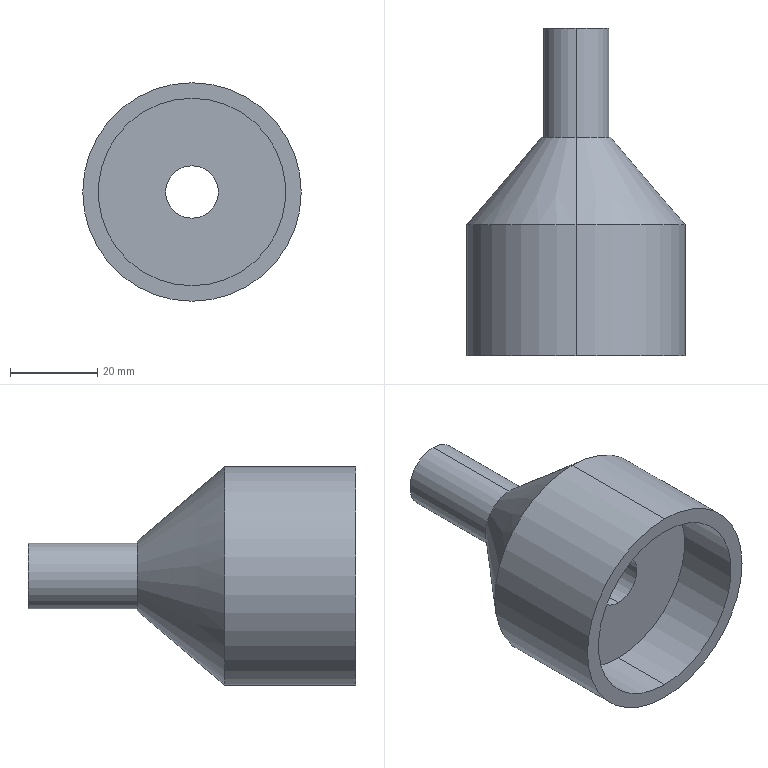Part | SolidWorks | features ICE 3, Chamfer 1, Extrusion 1 | 1 solid | 14 faces | box 50 x 75 x 50 mm | volume 53467 mm3 | cylinder 8 | plane 4 | cone 2 | commonest cylinder face diameters 12 x2 15 x2 42.907 x2 50 x2
STEP:
#1=CARTESIAN_POINT('',(0.,15.,21.453));
#2=VERTEX_POINT('',#1);
#3=CARTESIAN_POINT('',(0.,15.,-21.453));
#4=VERTEX_POINT('',#3);
#5=CARTESIAN_POINT('',(0.,15.,0.));
#6=DIRECTION('',(0.,-1.,0.));
#7=DIRECTION('',(0.,0.,-1.));
#8=AXIS2_PLACEMENT_3D('',#5,#6,#7);
#9=CIRCLE('',#8,21.453);
#10=EDGE_CURVE('',#2,#4,#9,.T.);
#11=ORIENTED_EDGE('',*,*,#10,.F.);
#12=CARTESIAN_POINT('',(0.,0.,21.453));
#13=VERTEX_POINT('',#12);
#14=CARTESIAN_POINT('',(0.,15.,21.453));
#15=DIRECTION('',(0.,-1.,0.));
#16=VECTOR('',#15,1000.);
#17=LINE('',#14,#16);
#18=EDGE_CURVE('',#2,#13,#17,.T.);
#19=ORIENTED_EDGE('',*,*,#18,.T.);
#20=CARTESIAN_POINT('',(0.,0.,-21.453));
#21=VERTEX_POINT('',#20);
#22=CARTESIAN_POINT('',(0.,0.,0.));
#23=DIRECTION('',(0.,-1.,0.));
#24=DIRECTION('',(0.,0.,-1.));
#25=AXIS2_PLACEMENT_3D('',#22,#23,#24);
#26=CIRCLE('',#25,21.453);
#27=EDGE_CURVE('',#13,#21,#26,.T.);
#28=ORIENTED_EDGE('',*,*,#27,.T.);
#29=CARTESIAN_POINT('',(0.,15.,-21.453));
#30=DIRECTION('',(0.,-1.,0.));
#31=VECTOR('',#30,1000.);
#32=LINE('',#29,#31);
#33=EDGE_CURVE('',#4,#21,#32,.T.);
#34=ORIENTED_EDGE('',*,*,#33,.F.);
#35=EDGE_LOOP('',(#11,#19,#28,#34));
#36=FACE_OUTER_BOUND('',#35,.T.);
#37=CARTESIAN_POINT('',(0.,15.,0.));
#38=DIRECTION('',(0.,-1.,0.));
#39=DIRECTION('',(0.,0.,-1.));
#40=AXIS2_PLACEMENT_3D('',#37,#38,#39);
#41=CYLINDRICAL_SURFACE('',#40,21.453);
#42=ADVANCED_FACE('',(#36),#41,.F.);
#43=CARTESIAN_POINT('',(0.,50.,8.));
#44=VERTEX_POINT('',#43);
#45=CARTESIAN_POINT('',(0.,50.,-8.));
#46=VERTEX_POINT('',#45);
#47=CARTESIAN_POINT('',(0.,50.,0.));
#48=DIRECTION('',(0.,1.,0.));
#49=DIRECTION('',(0.,0.,1.));
#50=AXIS2_PLACEMENT_3D('',#47,#48,#49);
#51=CIRCLE('',#50,8.);
#52=EDGE_CURVE('',#44,#46,#51,.T.);
#53=ORIENTED_EDGE('',*,*,#52,.F.);
#54=CARTESIAN_POINT('',(0.,30.,25.));
#55=VERTEX_POINT('',#54);
#56=CARTESIAN_POINT('',(0.,50.,8.));
#57=DIRECTION('',(0.,-0.7619,0.6476));
#58=VECTOR('',#57,1000.);
#59=LINE('',#56,#58);
#60=EDGE_CURVE('',#44,#55,#59,.T.);
#61=ORIENTED_EDGE('',*,*,#60,.T.);
#62=CARTESIAN_POINT('',(0.,30.,-25.));
#63=VERTEX_POINT('',#62);
#64=CARTESIAN_POINT('',(0.,30.,0.));
#65=DIRECTION('',(0.,-1.,0.));
#66=DIRECTION('',(0.,0.,1.));
#67=AXIS2_PLACEMENT_3D('',#64,#65,#66);
#68=CIRCLE('',#67,25.);
#69=EDGE_CURVE('',#63,#55,#68,.T.);
#70=ORIENTED_EDGE('',*,*,#69,.F.);
#71=CARTESIAN_POINT('',(0.,50.,-8.));
#72=DIRECTION('',(0.,-0.7619,-0.6476));
#73=VECTOR('',#72,1000.);
#74=LINE('',#71,#73);
#75=EDGE_CURVE('',#46,#63,#74,.T.);
#76=ORIENTED_EDGE('',*,*,#75,.F.);
#77=EDGE_LOOP('',(#53,#61,#70,#76));
#78=FACE_OUTER_BOUND('',#77,.T.);
#79=CARTESIAN_POINT('',(0.,50.,0.));
#80=DIRECTION('',(0.,-1.,0.));
#81=DIRECTION('',(0.,0.,-1.));
#82=AXIS2_PLACEMENT_3D('',#79,#80,#81);
#83=CONICAL_SURFACE('',#82,8.,0.7045);
#84=ADVANCED_FACE('',(#78),#83,.T.);
#85=CARTESIAN_POINT('',(0.,75.,7.5));
#86=VERTEX_POINT('',#85);
#87=CARTESIAN_POINT('',(0.,75.,-7.5));
#88=VERTEX_POINT('',#87);
#89=CARTESIAN_POINT('',(0.,75.,0.));
#90=DIRECTION('',(0.,1.,0.));
#91=DIRECTION('',(0.,0.,1.));
#92=AXIS2_PLACEMENT_3D('',#89,#90,#91);
#93=CIRCLE('',#92,7.5);
#94=EDGE_CURVE('',#86,#88,#93,.T.);
#95=ORIENTED_EDGE('',*,*,#94,.F.);
#96=CARTESIAN_POINT('',(0.,50.,7.5));
#97=VERTEX_POINT('',#96);
#98=CARTESIAN_POINT('',(0.,75.,7.5));
#99=DIRECTION('',(0.,-1.,0.));
#100=VECTOR('',#99,1000.);
#101=LINE('',#98,#100);
#102=EDGE_CURVE('',#86,#97,#101,.T.);
#103=ORIENTED_EDGE('',*,*,#102,.T.);
#104=CARTESIAN_POINT('',(0.,50.,-7.5));
#105=VERTEX_POINT('',#104);
#106=CARTESIAN_POINT('',(0.,50.,0.));
#107=DIRECTION('',(0.,1.,0.));
#108=DIRECTION('',(0.,0.,1.));
#109=AXIS2_PLACEMENT_3D('',#106,#107,#108);
#110=CIRCLE('',#109,7.5);
#111=EDGE_CURVE('',#97,#105,#110,.T.);
#112=ORIENTED_EDGE('',*,*,#111,.T.);
#113=CARTESIAN_POINT('',(0.,75.,-7.5));
#114=DIRECTION('',(0.,-1.,0.));
#115=VECTOR('',#114,1000.);
#116=LINE('',#113,#115);
#117=EDGE_CURVE('',#88,#105,#116,.T.);
#118=ORIENTED_EDGE('',*,*,#117,.F.);
#119=EDGE_LOOP('',(#95,#103,#112,#118));
#120=FACE_OUTER_BOUND('',#119,.T.);
#121=CARTESIAN_POINT('',(0.,75.,0.));
#122=DIRECTION('',(0.,-1.,0.));
#123=DIRECTION('',(0.,0.,-1.));
#124=AXIS2_PLACEMENT_3D('',#121,#122,#123);
#125=CYLINDRICAL_SURFACE('',#124,7.5);
#126=ADVANCED_FACE('',(#120),#125,.T.);
#127=ORIENTED_EDGE('',*,*,#69,.T.);
#128=CARTESIAN_POINT('',(0.,0.,25.));
#129=VERTEX_POINT('',#128);
#130=CARTESIAN_POINT('',(0.,50.,25.));
#131=DIRECTION('',(0.,-1.,0.));
#132=VECTOR('',#131,1000.);
#133=LINE('',#130,#132);
#134=EDGE_CURVE('',#55,#129,#133,.T.);
#135=ORIENTED_EDGE('',*,*,#134,.T.);
#136=CARTESIAN_POINT('',(0.,0.,-25.));
#137=VERTEX_POINT('',#136);
#138=CARTESIAN_POINT('',(0.,0.,0.));
#139=DIRECTION('',(0.,1.,0.));
#140=DIRECTION('',(0.,0.,1.));
#141=AXIS2_PLACEMENT_3D('',#138,#139,#140);
#142=CIRCLE('',#141,25.);
#143=EDGE_CURVE('',#129,#137,#142,.T.);
#144=ORIENTED_EDGE('',*,*,#143,.T.);
#145=CARTESIAN_POINT('',(0.,50.,-25.));
#146=DIRECTION('',(0.,-1.,0.));
#147=VECTOR('',#146,1000.);
#148=LINE('',#145,#147);
#149=EDGE_CURVE('',#63,#137,#148,.T.);
#150=ORIENTED_EDGE('',*,*,#149,.F.);
#151=EDGE_LOOP('',(#127,#135,#144,#150));
#152=FACE_OUTER_BOUND('',#151,.T.);
#153=CARTESIAN_POINT('',(0.,50.,0.));
#154=DIRECTION('',(0.,-1.,0.));
#155=DIRECTION('',(0.,0.,-1.));
#156=AXIS2_PLACEMENT_3D('',#153,#154,#155);
#157=CYLINDRICAL_SURFACE('',#156,25.);
#158=ADVANCED_FACE('',(#152),#157,.T.);
#159=CARTESIAN_POINT('',(0.,15.,-6.));
#160=VERTEX_POINT('',#159);
#161=CARTESIAN_POINT('',(0.,15.,6.));
#162=VERTEX_POINT('',#161);
#163=CARTESIAN_POINT('',(0.,15.,0.));
#164=DIRECTION('',(0.,1.,0.));
#165=DIRECTION('',(0.,0.,-1.));
#166=AXIS2_PLACEMENT_3D('',#163,#164,#165);
#167=CIRCLE('',#166,6.);
#168=EDGE_CURVE('',#160,#162,#167,.T.);
#169=ORIENTED_EDGE('',*,*,#168,.F.);
#170=CARTESIAN_POINT('',(0.,75.,-6.));
#171=VERTEX_POINT('',#170);
#172=CARTESIAN_POINT('',(0.,0.,-6.));
#173=DIRECTION('',(0.,1.,0.));
#174=VECTOR('',#173,1000.);
#175=LINE('',#172,#174);
#176=EDGE_CURVE('',#160,#171,#175,.T.);
#177=ORIENTED_EDGE('',*,*,#176,.T.);
#178=CARTESIAN_POINT('',(0.,75.,6.));
#179=VERTEX_POINT('',#178);
#180=CARTESIAN_POINT('',(0.,75.,0.));
#181=DIRECTION('',(0.,1.,0.));
#182=DIRECTION('',(0.,0.,1.));
#183=AXIS2_PLACEMENT_3D('',#180,#181,#182);
#184=CIRCLE('',#183,6.);
#185=EDGE_CURVE('',#171,#179,#184,.T.);
#186=ORIENTED_EDGE('',*,*,#185,.T.);
#187=CARTESIAN_POINT('',(0.,0.,6.));
#188=DIRECTION('',(0.,1.,0.));
#189=VECTOR('',#188,1000.);
#190=LINE('',#187,#189);
#191=EDGE_CURVE('',#162,#179,#190,.T.);
#192=ORIENTED_EDGE('',*,*,#191,.F.);
#193=EDGE_LOOP('',(#169,#177,#186,#192));
#194=FACE_OUTER_BOUND('',#193,.T.);
#195=CARTESIAN_POINT('',(0.,0.,0.));
#196=DIRECTION('',(0.,1.,0.));
#197=DIRECTION('',(0.,0.,1.));
#198=AXIS2_PLACEMENT_3D('',#195,#196,#197);
#199=CYLINDRICAL_SURFACE('',#198,6.);
#200=ADVANCED_FACE('',(#194),#199,.F.);
#201=ORIENTED_EDGE('',*,*,#176,.F.);
#202=CARTESIAN_POINT('',(0.,15.,0.));
#203=DIRECTION('',(0.,1.,0.));
#204=DIRECTION('',(0.,0.,-1.));
#205=AXIS2_PLACEMENT_3D('',#202,#203,#204);
#206=CIRCLE('',#205,6.);
#207=EDGE_CURVE('',#162,#160,#206,.T.);
#208=ORIENTED_EDGE('',*,*,#207,.F.);
#209=ORIENTED_EDGE('',*,*,#191,.T.);
#210=CARTESIAN_POINT('',(0.,75.,0.));
#211=DIRECTION('',(0.,1.,0.));
#212=DIRECTION('',(0.,0.,1.));
#213=AXIS2_PLACEMENT_3D('',#210,#211,#212);
#214=CIRCLE('',#213,6.);
#215=EDGE_CURVE('',#179,#171,#214,.T.);
#216=ORIENTED_EDGE('',*,*,#215,.T.);
#217=EDGE_LOOP('',(#201,#208,#209,#216));
#218=FACE_OUTER_BOUND('',#217,.T.);
#219=CARTESIAN_POINT('',(0.,0.,0.));
#220=DIRECTION('',(0.,1.,0.));
#221=DIRECTION('',(0.,0.,1.));
#222=AXIS2_PLACEMENT_3D('',#219,#220,#221);
#223=CYLINDRICAL_SURFACE('',#222,6.);
#224=ADVANCED_FACE('',(#218),#223,.F.);
#225=ORIENTED_EDGE('',*,*,#134,.F.);
#226=CARTESIAN_POINT('',(0.,30.,0.));
#227=DIRECTION('',(0.,-1.,0.));
#228=DIRECTION('',(0.,0.,1.));
#229=AXIS2_PLACEMENT_3D('',#226,#227,#228);
#230=CIRCLE('',#229,25.);
#231=EDGE_CURVE('',#55,#63,#230,.T.);
#232=ORIENTED_EDGE('',*,*,#231,.T.);
#233=ORIENTED_EDGE('',*,*,#149,.T.);
#234=CARTESIAN_POINT('',(0.,0.,0.));
#235=DIRECTION('',(0.,1.,0.));
#236=DIRECTION('',(0.,0.,1.));
#237=AXIS2_PLACEMENT_3D('',#234,#235,#236);
#238=CIRCLE('',#237,25.);
#239=EDGE_CURVE('',#137,#129,#238,.T.);
#240=ORIENTED_EDGE('',*,*,#239,.T.);
#241=EDGE_LOOP('',(#225,#232,#233,#240));
#242=FACE_OUTER_BOUND('',#241,.T.);
#243=CARTESIAN_POINT('',(0.,50.,0.));
#244=DIRECTION('',(0.,-1.,0.));
#245=DIRECTION('',(0.,0.,-1.));
#246=AXIS2_PLACEMENT_3D('',#243,#244,#245);
#247=CYLINDRICAL_SURFACE('',#246,25.);
#248=ADVANCED_FACE('',(#242),#247,.T.);
#249=CARTESIAN_POINT('',(0.,50.,0.));
#250=DIRECTION('',(0.,1.,0.));
#251=DIRECTION('',(0.,0.,1.));
#252=AXIS2_PLACEMENT_3D('',#249,#250,#251);
#253=CIRCLE('',#252,8.);
#254=EDGE_CURVE('',#46,#44,#253,.T.);
#255=ORIENTED_EDGE('',*,*,#254,.T.);
#256=ORIENTED_EDGE('',*,*,#52,.T.);
#257=EDGE_LOOP('',(#255,#256));
#258=FACE_OUTER_BOUND('',#257,.T.);
#259=CARTESIAN_POINT('',(0.,50.,0.));
#260=DIRECTION('',(0.,1.,0.));
#261=DIRECTION('',(0.,0.,1.));
#262=AXIS2_PLACEMENT_3D('',#259,#260,#261);
#263=CIRCLE('',#262,7.5);
#264=EDGE_CURVE('',#105,#97,#263,.T.);
#265=ORIENTED_EDGE('',*,*,#264,.F.);
#266=ORIENTED_EDGE('',*,*,#111,.F.);
#267=EDGE_LOOP('',(#265,#266));
#268=FACE_BOUND('',#267,.T.);
#269=CARTESIAN_POINT('',(0.,50.,0.));
#270=DIRECTION('',(0.,1.,0.));
#271=DIRECTION('',(0.,0.,1.));
#272=AXIS2_PLACEMENT_3D('',#269,#270,#271);
#273=PLANE('',#272);
#274=ADVANCED_FACE('',(#258,#268),#273,.T.);
#275=CARTESIAN_POINT('',(0.,0.,0.));
#276=DIRECTION('',(0.,-1.,0.));
#277=DIRECTION('',(0.,0.,-1.));
#278=AXIS2_PLACEMENT_3D('',#275,#276,#277);
#279=CIRCLE('',#278,21.453);
#280=EDGE_CURVE('',#21,#13,#279,.T.);
#281=ORIENTED_EDGE('',*,*,#280,.F.);
#282=ORIENTED_EDGE('',*,*,#27,.F.);
#283=EDGE_LOOP('',(#281,#282));
#284=FACE_BOUND('',#283,.T.);
#285=ORIENTED_EDGE('',*,*,#239,.F.);
#286=ORIENTED_EDGE('',*,*,#143,.F.);
#287=EDGE_LOOP('',(#285,#286));
#288=FACE_OUTER_BOUND('',#287,.T.);
#289=CARTESIAN_POINT('',(0.,0.,0.));
#290=DIRECTION('',(0.,1.,0.));
#291=DIRECTION('',(0.,0.,1.));
#292=AXIS2_PLACEMENT_3D('',#289,#290,#291);
#293=PLANE('',#292);
#294=ADVANCED_FACE('',(#284,#288),#293,.F.);
#295=ORIENTED_EDGE('',*,*,#102,.F.);
#296=CARTESIAN_POINT('',(0.,75.,0.));
#297=DIRECTION('',(0.,1.,0.));
#298=DIRECTION('',(0.,0.,1.));
#299=AXIS2_PLACEMENT_3D('',#296,#297,#298);
#300=CIRCLE('',#299,7.5);
#301=EDGE_CURVE('',#88,#86,#300,.T.);
#302=ORIENTED_EDGE('',*,*,#301,.F.);
#303=ORIENTED_EDGE('',*,*,#117,.T.);
#304=ORIENTED_EDGE('',*,*,#264,.T.);
#305=EDGE_LOOP('',(#295,#302,#303,#304));
#306=FACE_OUTER_BOUND('',#305,.T.);
#307=CARTESIAN_POINT('',(0.,75.,0.));
#308=DIRECTION('',(0.,-1.,0.));
#309=DIRECTION('',(0.,0.,-1.));
#310=AXIS2_PLACEMENT_3D('',#307,#308,#309);
#311=CYLINDRICAL_SURFACE('',#310,7.5);
#312=ADVANCED_FACE('',(#306),#311,.T.);
#313=ORIENTED_EDGE('',*,*,#215,.F.);
#314=ORIENTED_EDGE('',*,*,#185,.F.);
#315=EDGE_LOOP('',(#313,#314));
#316=FACE_BOUND('',#315,.T.);
#317=ORIENTED_EDGE('',*,*,#301,.T.);
#318=ORIENTED_EDGE('',*,*,#94,.T.);
#319=EDGE_LOOP('',(#317,#318));
#320=FACE_OUTER_BOUND('',#319,.T.);
#321=CARTESIAN_POINT('',(0.,75.,0.));
#322=DIRECTION('',(0.,1.,0.));
#323=DIRECTION('',(0.,0.,1.));
#324=AXIS2_PLACEMENT_3D('',#321,#322,#323);
#325=PLANE('',#324);
#326=ADVANCED_FACE('',(#316,#320),#325,.T.);
#327=ORIENTED_EDGE('',*,*,#60,.F.);
#328=ORIENTED_EDGE('',*,*,#254,.F.);
#329=ORIENTED_EDGE('',*,*,#75,.T.);
#330=ORIENTED_EDGE('',*,*,#231,.F.);
#331=EDGE_LOOP('',(#327,#328,#329,#330));
#332=FACE_OUTER_BOUND('',#331,.T.);
#333=CARTESIAN_POINT('',(0.,50.,0.));
#334=DIRECTION('',(0.,-1.,0.));
#335=DIRECTION('',(0.,0.,-1.));
#336=AXIS2_PLACEMENT_3D('',#333,#334,#335);
#337=CONICAL_SURFACE('',#336,8.,0.7045);
#338=ADVANCED_FACE('',(#332),#337,.T.);
#339=CARTESIAN_POINT('',(0.,15.,0.));
#340=DIRECTION('',(0.,-1.,0.));
#341=DIRECTION('',(0.,0.,-1.));
#342=AXIS2_PLACEMENT_3D('',#339,#340,#341);
#343=CIRCLE('',#342,21.453);
#344=EDGE_CURVE('',#4,#2,#343,.T.);
#345=ORIENTED_EDGE('',*,*,#344,.T.);
#346=ORIENTED_EDGE('',*,*,#10,.T.);
#347=EDGE_LOOP('',(#345,#346));
#348=FACE_OUTER_BOUND('',#347,.T.);
#349=ORIENTED_EDGE('',*,*,#207,.T.);
#350=ORIENTED_EDGE('',*,*,#168,.T.);
#351=EDGE_LOOP('',(#349,#350));
#352=FACE_BOUND('',#351,.T.);
#353=CARTESIAN_POINT('',(0.,15.,0.));
#354=DIRECTION('',(0.,-1.,0.));
#355=DIRECTION('',(0.,0.,-1.));
#356=AXIS2_PLACEMENT_3D('',#353,#354,#355);
#357=PLANE('',#356);
#358=ADVANCED_FACE('',(#348,#352),#357,.T.);
#359=ORIENTED_EDGE('',*,*,#18,.F.);
#360=ORIENTED_EDGE('',*,*,#344,.F.);
#361=ORIENTED_EDGE('',*,*,#33,.T.);
#362=ORIENTED_EDGE('',*,*,#280,.T.);
#363=EDGE_LOOP('',(#359,#360,#361,#362));
#364=FACE_OUTER_BOUND('',#363,.T.);
#365=CARTESIAN_POINT('',(0.,15.,0.));
#366=DIRECTION('',(0.,-1.,0.));
#367=DIRECTION('',(0.,0.,-1.));
#368=AXIS2_PLACEMENT_3D('',#365,#366,#367);
#369=CYLINDRICAL_SURFACE('',#368,21.453);
#370=ADVANCED_FACE('',(#364),#369,.F.);
#371=CLOSED_SHELL('',(#42,#84,#126,#158,#200,#224,#248,#274,#294,#312,#326,#338,#358,#370));
#372=MANIFOLD_SOLID_BREP('',#371);
#373=CARTESIAN_POINT('',(0.,0.,0.));
#374=DIRECTION('',(0.,0.,1.));
#375=DIRECTION('',(1.,0.,0.));
#376=AXIS2_PLACEMENT_3D('',#373,#374,#375);
#377=(LENGTH_UNIT()NAMED_UNIT(*)SI_UNIT(.MILLI.,.METRE.));
#378=UNCERTAINTY_MEASURE_WITH_UNIT(LENGTH_MEASURE(0.00001),#377,'','');
#379=(NAMED_UNIT(*)PLANE_ANGLE_UNIT()SI_UNIT($,.RADIAN.));
#380=(NAMED_UNIT(*)SI_UNIT($,.STERADIAN.)SOLID_ANGLE_UNIT());
#381=(GEOMETRIC_REPRESENTATION_CONTEXT(3)GLOBAL_UNCERTAINTY_ASSIGNED_CONTEXT((#378))GLOBAL_UNIT_ASSIGNED_CONTEXT((#377,#379,#380))REPRESENTATION_CONTEXT('',''));
#382=ADVANCED_BREP_SHAPE_REPRESENTATION('',(#372,#376),#381);